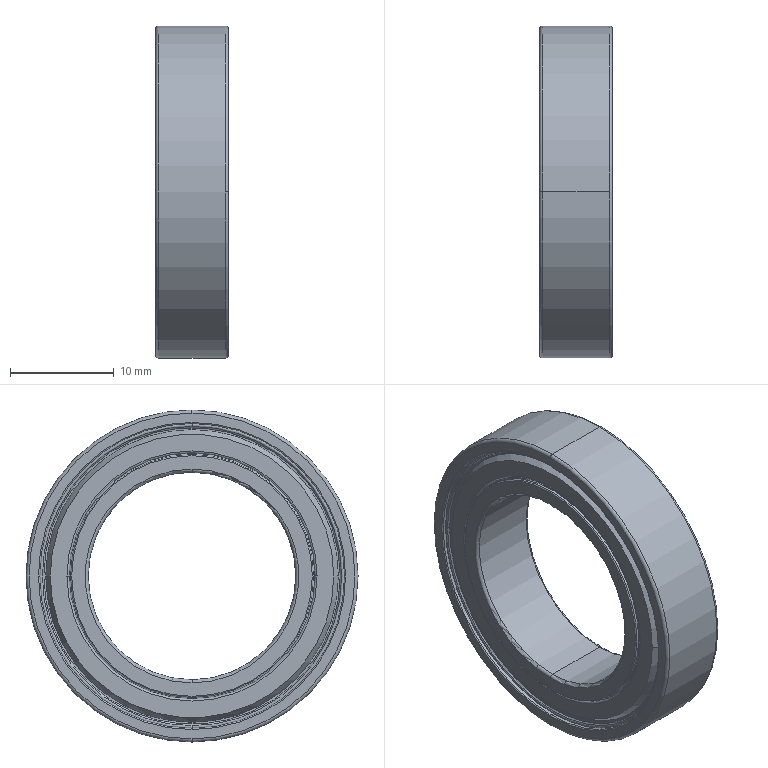Part | SolidWorks | features BaseBody 1 | 1 solid | 134 faces | box 7 x 32 x 32 mm | volume 2844 mm3 | torus 50 | cone 40 | cylinder 32 | plane 12 | commonest cylinder face diameters 22.7 x4 23.4 x4 23.7 x4 24 x4 24.1 x4 28 x4